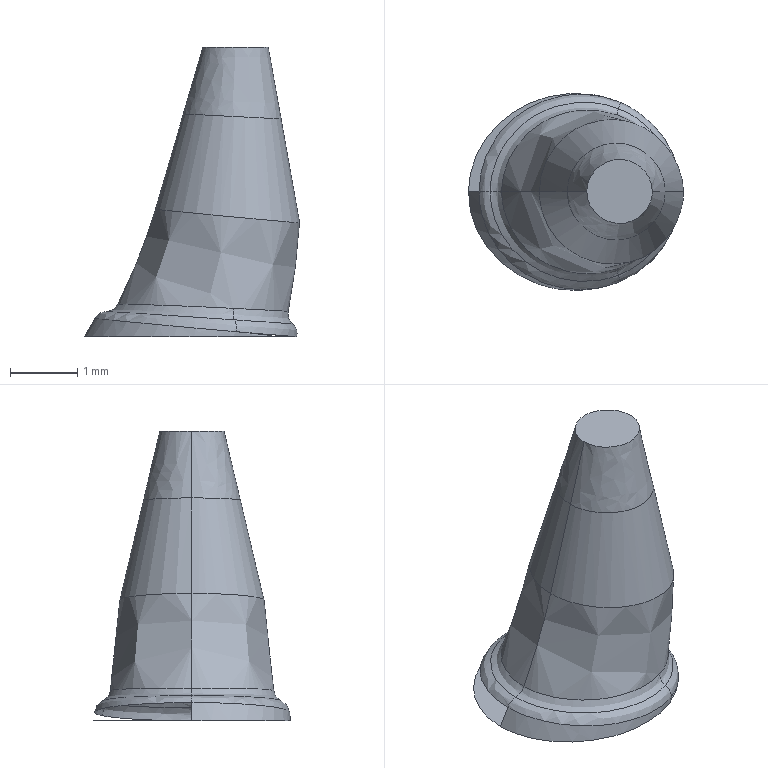Part | STEP file | solid 213 | 1 solid | 18 faces | box 3.206 x 2.939 x 4.314 mm | volume 13.64 mm3 | spline 16 | plane 2